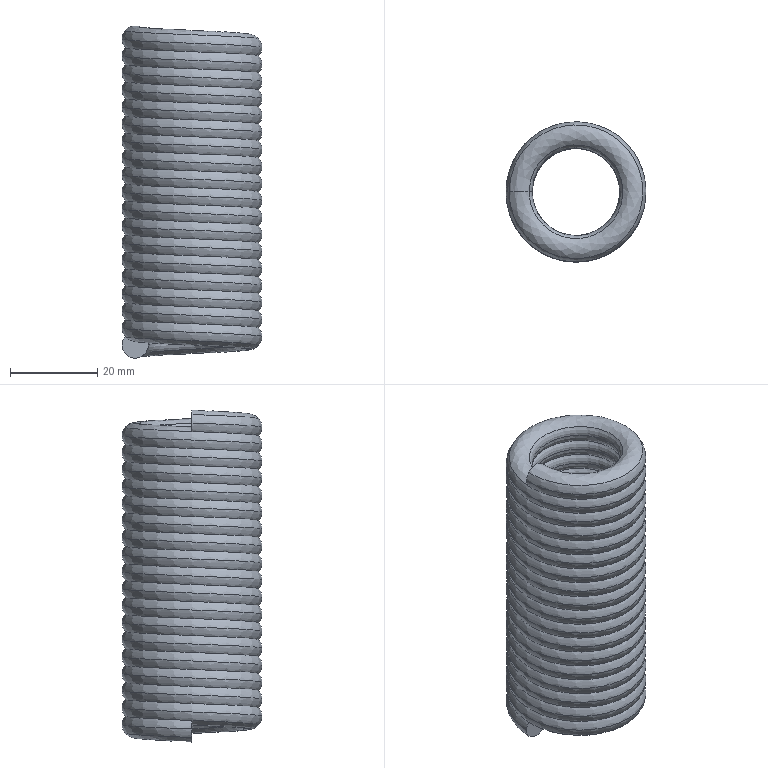Part | SolidWorks | features Helix 1, Sweep 1 | 1 solid | 8 faces | box 32 x 32 x 76 mm | volume 32270 mm3 | spline 6 | plane 2